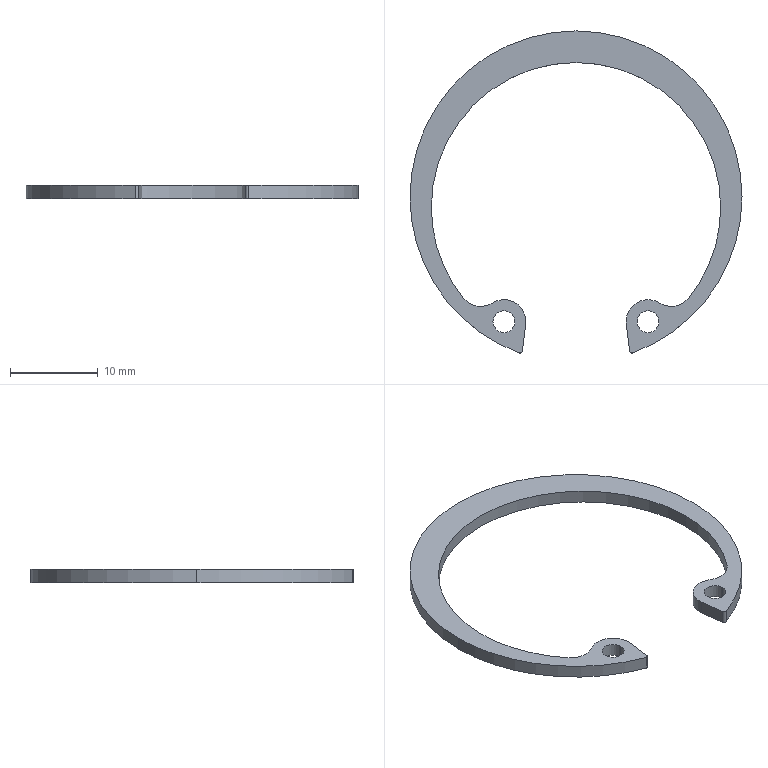Part | STEP file | TBP51-35 | 1 solid | 21 faces | box 37.8 x 36.681 x 1.5 mm | volume 416.093 mm3 | cylinder 17 | plane 4 | commonest cylinder face diameters 5 x5 2.5 x4 32.95 x3 37.8 x3 0.5 x2